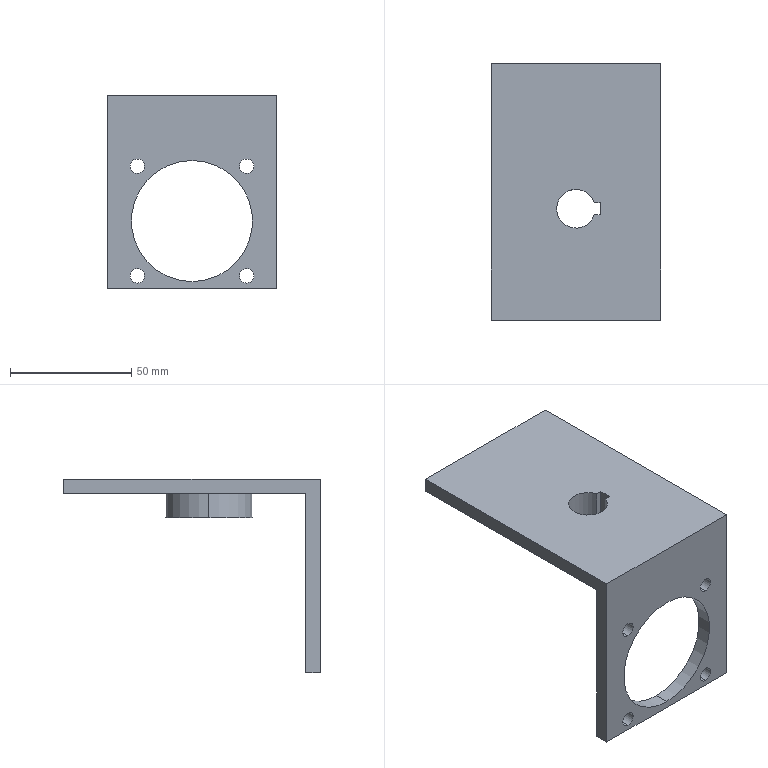Part | SolidWorks | features ICE 3, Cut 1, Extrusion 1 | 1 solid | 26 faces | box 70 x 106 x 80 mm | volume 69922 mm3 | cylinder 14 | plane 12 | commonest cylinder face diameters 6 x6 6.013 x2 16 x2 36 x2 50.018 x2
STEP:
#1=CARTESIAN_POINT('',(22.627,-46.,-71.627));
#2=VERTEX_POINT('',#1);
#3=CARTESIAN_POINT('',(22.627,-46.,-65.627));
#4=VERTEX_POINT('',#3);
#5=CARTESIAN_POINT('',(22.627,-46.,-68.627));
#6=DIRECTION('',(0.,1.,0.));
#7=DIRECTION('',(0.,0.,1.));
#8=AXIS2_PLACEMENT_3D('',#5,#6,#7);
#9=CIRCLE('',#8,3.);
#10=EDGE_CURVE('',#2,#4,#9,.T.);
#11=ORIENTED_EDGE('',*,*,#10,.F.);
#12=CARTESIAN_POINT('',(22.627,-40.,-71.627));
#13=VERTEX_POINT('',#12);
#14=CARTESIAN_POINT('',(22.627,-46.,-71.627));
#15=DIRECTION('',(0.,1.,0.));
#16=VECTOR('',#15,1000.);
#17=LINE('',#14,#16);
#18=EDGE_CURVE('',#2,#13,#17,.T.);
#19=ORIENTED_EDGE('',*,*,#18,.T.);
#20=CARTESIAN_POINT('',(22.627,-40.,-65.627));
#21=VERTEX_POINT('',#20);
#22=CARTESIAN_POINT('',(22.627,-40.,-68.627));
#23=DIRECTION('',(0.,1.,0.));
#24=DIRECTION('',(0.,0.,1.));
#25=AXIS2_PLACEMENT_3D('',#22,#23,#24);
#26=CIRCLE('',#25,3.);
#27=EDGE_CURVE('',#13,#21,#26,.T.);
#28=ORIENTED_EDGE('',*,*,#27,.T.);
#29=CARTESIAN_POINT('',(22.627,-46.,-65.627));
#30=DIRECTION('',(0.,1.,0.));
#31=VECTOR('',#30,1000.);
#32=LINE('',#29,#31);
#33=EDGE_CURVE('',#4,#21,#32,.T.);
#34=ORIENTED_EDGE('',*,*,#33,.F.);
#35=EDGE_LOOP('',(#11,#19,#28,#34));
#36=FACE_OUTER_BOUND('',#35,.T.);
#37=CARTESIAN_POINT('',(22.627,-46.,-68.627));
#38=DIRECTION('',(0.,1.,0.));
#39=DIRECTION('',(0.,0.,1.));
#40=AXIS2_PLACEMENT_3D('',#37,#38,#39);
#41=CYLINDRICAL_SURFACE('',#40,3.);
#42=ADVANCED_FACE('',(#36),#41,.F.);
#43=CARTESIAN_POINT('',(22.627,-46.,-26.373));
#44=VERTEX_POINT('',#43);
#45=CARTESIAN_POINT('',(22.627,-46.,-20.373));
#46=VERTEX_POINT('',#45);
#47=CARTESIAN_POINT('',(22.627,-46.,-23.373));
#48=DIRECTION('',(0.,1.,0.));
#49=DIRECTION('',(0.,0.,1.));
#50=AXIS2_PLACEMENT_3D('',#47,#48,#49);
#51=CIRCLE('',#50,3.);
#52=EDGE_CURVE('',#44,#46,#51,.T.);
#53=ORIENTED_EDGE('',*,*,#52,.F.);
#54=CARTESIAN_POINT('',(22.627,-40.,-26.373));
#55=VERTEX_POINT('',#54);
#56=CARTESIAN_POINT('',(22.627,-46.,-26.373));
#57=DIRECTION('',(0.,1.,0.));
#58=VECTOR('',#57,1000.);
#59=LINE('',#56,#58);
#60=EDGE_CURVE('',#44,#55,#59,.T.);
#61=ORIENTED_EDGE('',*,*,#60,.T.);
#62=CARTESIAN_POINT('',(22.627,-40.,-20.373));
#63=VERTEX_POINT('',#62);
#64=CARTESIAN_POINT('',(22.627,-40.,-23.373));
#65=DIRECTION('',(0.,1.,0.));
#66=DIRECTION('',(0.,0.,1.));
#67=AXIS2_PLACEMENT_3D('',#64,#65,#66);
#68=CIRCLE('',#67,3.);
#69=EDGE_CURVE('',#55,#63,#68,.T.);
#70=ORIENTED_EDGE('',*,*,#69,.T.);
#71=CARTESIAN_POINT('',(22.627,-46.,-20.373));
#72=DIRECTION('',(0.,1.,0.));
#73=VECTOR('',#72,1000.);
#74=LINE('',#71,#73);
#75=EDGE_CURVE('',#46,#63,#74,.T.);
#76=ORIENTED_EDGE('',*,*,#75,.F.);
#77=EDGE_LOOP('',(#53,#61,#70,#76));
#78=FACE_OUTER_BOUND('',#77,.T.);
#79=CARTESIAN_POINT('',(22.627,-46.,-23.373));
#80=DIRECTION('',(0.,1.,0.));
#81=DIRECTION('',(0.,0.,1.));
#82=AXIS2_PLACEMENT_3D('',#79,#80,#81);
#83=CYLINDRICAL_SURFACE('',#82,3.);
#84=ADVANCED_FACE('',(#78),#83,.F.);
#85=CARTESIAN_POINT('',(-0.009138,-46.,-71.009));
#86=VERTEX_POINT('',#85);
#87=CARTESIAN_POINT('',(-0.009138,-46.,-20.991));
#88=VERTEX_POINT('',#87);
#89=CARTESIAN_POINT('',(-0.009138,-46.,-46.));
#90=DIRECTION('',(0.,1.,0.));
#91=DIRECTION('',(0.,0.,1.));
#92=AXIS2_PLACEMENT_3D('',#89,#90,#91);
#93=CIRCLE('',#92,25.009);
#94=EDGE_CURVE('',#86,#88,#93,.T.);
#95=ORIENTED_EDGE('',*,*,#94,.F.);
#96=CARTESIAN_POINT('',(-0.009138,-40.,-71.009));
#97=VERTEX_POINT('',#96);
#98=CARTESIAN_POINT('',(-0.009138,-46.,-71.009));
#99=DIRECTION('',(0.,1.,0.));
#100=VECTOR('',#99,1000.);
#101=LINE('',#98,#100);
#102=EDGE_CURVE('',#86,#97,#101,.T.);
#103=ORIENTED_EDGE('',*,*,#102,.T.);
#104=CARTESIAN_POINT('',(-0.009138,-40.,-20.991));
#105=VERTEX_POINT('',#104);
#106=CARTESIAN_POINT('',(-0.009138,-40.,-46.));
#107=DIRECTION('',(0.,1.,0.));
#108=DIRECTION('',(0.,0.,1.));
#109=AXIS2_PLACEMENT_3D('',#106,#107,#108);
#110=CIRCLE('',#109,25.009);
#111=EDGE_CURVE('',#97,#105,#110,.T.);
#112=ORIENTED_EDGE('',*,*,#111,.T.);
#113=CARTESIAN_POINT('',(-0.009138,-46.,-20.991));
#114=DIRECTION('',(0.,1.,0.));
#115=VECTOR('',#114,1000.);
#116=LINE('',#113,#115);
#117=EDGE_CURVE('',#88,#105,#116,.T.);
#118=ORIENTED_EDGE('',*,*,#117,.F.);
#119=EDGE_LOOP('',(#95,#103,#112,#118));
#120=FACE_OUTER_BOUND('',#119,.T.);
#121=CARTESIAN_POINT('',(-0.009138,-46.,-46.));
#122=DIRECTION('',(0.,1.,0.));
#123=DIRECTION('',(0.,0.,1.));
#124=AXIS2_PLACEMENT_3D('',#121,#122,#123);
#125=CYLINDRICAL_SURFACE('',#124,25.009);
#126=ADVANCED_FACE('',(#120),#125,.F.);
#127=CARTESIAN_POINT('',(-22.627,-46.,-26.373));
#128=VERTEX_POINT('',#127);
#129=CARTESIAN_POINT('',(-22.627,-46.,-20.373));
#130=VERTEX_POINT('',#129);
#131=CARTESIAN_POINT('',(-22.627,-46.,-23.373));
#132=DIRECTION('',(0.,1.,0.));
#133=DIRECTION('',(0.,0.,1.));
#134=AXIS2_PLACEMENT_3D('',#131,#132,#133);
#135=CIRCLE('',#134,3.);
#136=EDGE_CURVE('',#128,#130,#135,.T.);
#137=ORIENTED_EDGE('',*,*,#136,.F.);
#138=CARTESIAN_POINT('',(-22.627,-40.,-26.373));
#139=VERTEX_POINT('',#138);
#140=CARTESIAN_POINT('',(-22.627,-46.,-26.373));
#141=DIRECTION('',(0.,1.,0.));
#142=VECTOR('',#141,1000.);
#143=LINE('',#140,#142);
#144=EDGE_CURVE('',#128,#139,#143,.T.);
#145=ORIENTED_EDGE('',*,*,#144,.T.);
#146=CARTESIAN_POINT('',(-22.627,-40.,-20.373));
#147=VERTEX_POINT('',#146);
#148=CARTESIAN_POINT('',(-22.627,-40.,-23.373));
#149=DIRECTION('',(0.,1.,0.));
#150=DIRECTION('',(0.,0.,1.));
#151=AXIS2_PLACEMENT_3D('',#148,#149,#150);
#152=CIRCLE('',#151,3.);
#153=EDGE_CURVE('',#139,#147,#152,.T.);
#154=ORIENTED_EDGE('',*,*,#153,.T.);
#155=CARTESIAN_POINT('',(-22.627,-46.,-20.373));
#156=DIRECTION('',(0.,1.,0.));
#157=VECTOR('',#156,1000.);
#158=LINE('',#155,#157);
#159=EDGE_CURVE('',#130,#147,#158,.T.);
#160=ORIENTED_EDGE('',*,*,#159,.F.);
#161=EDGE_LOOP('',(#137,#145,#154,#160));
#162=FACE_OUTER_BOUND('',#161,.T.);
#163=CARTESIAN_POINT('',(-22.627,-46.,-23.373));
#164=DIRECTION('',(0.,1.,0.));
#165=DIRECTION('',(0.,0.,1.));
#166=AXIS2_PLACEMENT_3D('',#163,#164,#165);
#167=CYLINDRICAL_SURFACE('',#166,3.);
#168=ADVANCED_FACE('',(#162),#167,.F.);
#169=CARTESIAN_POINT('',(-22.627,-46.,-71.634));
#170=VERTEX_POINT('',#169);
#171=CARTESIAN_POINT('',(-22.627,-46.,-65.621));
#172=VERTEX_POINT('',#171);
#173=CARTESIAN_POINT('',(-22.627,-46.,-68.627));
#174=DIRECTION('',(0.,1.,0.));
#175=DIRECTION('',(0.,0.,1.));
#176=AXIS2_PLACEMENT_3D('',#173,#174,#175);
#177=CIRCLE('',#176,3.006);
#178=EDGE_CURVE('',#170,#172,#177,.T.);
#179=ORIENTED_EDGE('',*,*,#178,.F.);
#180=CARTESIAN_POINT('',(-22.627,-40.,-71.634));
#181=VERTEX_POINT('',#180);
#182=CARTESIAN_POINT('',(-22.627,-46.,-71.634));
#183=DIRECTION('',(0.,1.,0.));
#184=VECTOR('',#183,1000.);
#185=LINE('',#182,#184);
#186=EDGE_CURVE('',#170,#181,#185,.T.);
#187=ORIENTED_EDGE('',*,*,#186,.T.);
#188=CARTESIAN_POINT('',(-22.627,-40.,-65.621));
#189=VERTEX_POINT('',#188);
#190=CARTESIAN_POINT('',(-22.627,-40.,-68.627));
#191=DIRECTION('',(0.,1.,0.));
#192=DIRECTION('',(0.,0.,1.));
#193=AXIS2_PLACEMENT_3D('',#190,#191,#192);
#194=CIRCLE('',#193,3.006);
#195=EDGE_CURVE('',#181,#189,#194,.T.);
#196=ORIENTED_EDGE('',*,*,#195,.T.);
#197=CARTESIAN_POINT('',(-22.627,-46.,-65.621));
#198=DIRECTION('',(0.,1.,0.));
#199=VECTOR('',#198,1000.);
#200=LINE('',#197,#199);
#201=EDGE_CURVE('',#172,#189,#200,.T.);
#202=ORIENTED_EDGE('',*,*,#201,.F.);
#203=EDGE_LOOP('',(#179,#187,#196,#202));
#204=FACE_OUTER_BOUND('',#203,.T.);
#205=CARTESIAN_POINT('',(-22.627,-46.,-68.627));
#206=DIRECTION('',(0.,1.,0.));
#207=DIRECTION('',(0.,0.,1.));
#208=AXIS2_PLACEMENT_3D('',#205,#206,#207);
#209=CYLINDRICAL_SURFACE('',#208,3.006);
#210=ADVANCED_FACE('',(#204),#209,.F.);
#211=CARTESIAN_POINT('',(-18.,0.,-10.));
#212=VERTEX_POINT('',#211);
#213=CARTESIAN_POINT('',(18.,0.,-10.));
#214=VERTEX_POINT('',#213);
#215=CARTESIAN_POINT('',(0.,0.,-10.));
#216=DIRECTION('',(0.,0.,-1.));
#217=DIRECTION('',(-1.,0.,0.));
#218=AXIS2_PLACEMENT_3D('',#215,#216,#217);
#219=CIRCLE('',#218,18.);
#220=EDGE_CURVE('',#212,#214,#219,.T.);
#221=ORIENTED_EDGE('',*,*,#220,.F.);
#222=CARTESIAN_POINT('',(-18.,0.,0.));
#223=VERTEX_POINT('',#222);
#224=CARTESIAN_POINT('',(-18.,0.,-10.));
#225=DIRECTION('',(0.,0.,1.));
#226=VECTOR('',#225,1000.);
#227=LINE('',#224,#226);
#228=EDGE_CURVE('',#212,#223,#227,.T.);
#229=ORIENTED_EDGE('',*,*,#228,.T.);
#230=CARTESIAN_POINT('',(18.,0.,0.));
#231=VERTEX_POINT('',#230);
#232=CARTESIAN_POINT('',(0.,0.,0.));
#233=DIRECTION('',(0.,0.,-1.));
#234=DIRECTION('',(1.,0.,0.));
#235=AXIS2_PLACEMENT_3D('',#232,#233,#234);
#236=CIRCLE('',#235,18.);
#237=EDGE_CURVE('',#223,#231,#236,.T.);
#238=ORIENTED_EDGE('',*,*,#237,.T.);
#239=CARTESIAN_POINT('',(18.,0.,-10.));
#240=DIRECTION('',(0.,0.,1.));
#241=VECTOR('',#240,1000.);
#242=LINE('',#239,#241);
#243=EDGE_CURVE('',#214,#231,#242,.T.);
#244=ORIENTED_EDGE('',*,*,#243,.F.);
#245=EDGE_LOOP('',(#221,#229,#238,#244));
#246=FACE_OUTER_BOUND('',#245,.T.);
#247=CARTESIAN_POINT('',(0.,0.,-10.));
#248=DIRECTION('',(0.,0.,1.));
#249=DIRECTION('',(1.,0.,0.));
#250=AXIS2_PLACEMENT_3D('',#247,#248,#249);
#251=CYLINDRICAL_SURFACE('',#250,18.);
#252=ADVANCED_FACE('',(#246),#251,.T.);
#253=CARTESIAN_POINT('',(7.599,2.5,6.));
#254=VERTEX_POINT('',#253);
#255=CARTESIAN_POINT('',(-8.,0.,6.));
#256=VERTEX_POINT('',#255);
#257=CARTESIAN_POINT('',(0.,0.,6.));
#258=DIRECTION('',(0.,0.,1.));
#259=DIRECTION('',(1.,0.,0.));
#260=AXIS2_PLACEMENT_3D('',#257,#258,#259);
#261=CIRCLE('',#260,8.);
#262=EDGE_CURVE('',#254,#256,#261,.T.);
#263=ORIENTED_EDGE('',*,*,#262,.T.);
#264=CARTESIAN_POINT('',(-8.,0.,-10.));
#265=VERTEX_POINT('',#264);
#266=CARTESIAN_POINT('',(-8.,0.,6.));
#267=DIRECTION('',(0.,0.,-1.));
#268=VECTOR('',#267,1000.);
#269=LINE('',#266,#268);
#270=EDGE_CURVE('',#256,#265,#269,.T.);
#271=ORIENTED_EDGE('',*,*,#270,.T.);
#272=CARTESIAN_POINT('',(7.599,2.5,-10.));
#273=VERTEX_POINT('',#272);
#274=CARTESIAN_POINT('',(0.,0.,-10.));
#275=DIRECTION('',(0.,0.,-1.));
#276=DIRECTION('',(-1.,0.,0.));
#277=AXIS2_PLACEMENT_3D('',#274,#275,#276);
#278=CIRCLE('',#277,8.);
#279=EDGE_CURVE('',#265,#273,#278,.T.);
#280=ORIENTED_EDGE('',*,*,#279,.T.);
#281=CARTESIAN_POINT('',(7.599,2.5,6.));
#282=DIRECTION('',(0.,0.,-1.));
#283=VECTOR('',#282,1000.);
#284=LINE('',#281,#283);
#285=EDGE_CURVE('',#254,#273,#284,.T.);
#286=ORIENTED_EDGE('',*,*,#285,.F.);
#287=EDGE_LOOP('',(#263,#271,#280,#286));
#288=FACE_OUTER_BOUND('',#287,.T.);
#289=CARTESIAN_POINT('',(0.,0.,6.));
#290=DIRECTION('',(0.,0.,-1.));
#291=DIRECTION('',(-1.,0.,0.));
#292=AXIS2_PLACEMENT_3D('',#289,#290,#291);
#293=CYLINDRICAL_SURFACE('',#292,8.);
#294=ADVANCED_FACE('',(#288),#293,.F.);
#295=CARTESIAN_POINT('',(-35.,60.,0.));
#296=VERTEX_POINT('',#295);
#297=CARTESIAN_POINT('',(-35.,-40.,0.));
#298=VERTEX_POINT('',#297);
#299=CARTESIAN_POINT('',(-35.,60.,0.));
#300=DIRECTION('',(0.,-1.,0.));
#301=VECTOR('',#300,1000.);
#302=LINE('',#299,#301);
#303=EDGE_CURVE('',#296,#298,#302,.T.);
#304=ORIENTED_EDGE('',*,*,#303,.F.);
#305=CARTESIAN_POINT('',(35.,60.,0.));
#306=VERTEX_POINT('',#305);
#307=CARTESIAN_POINT('',(-35.,60.,0.));
#308=DIRECTION('',(-1.,0.,0.));
#309=VECTOR('',#308,1000.);
#310=LINE('',#307,#309);
#311=EDGE_CURVE('',#306,#296,#310,.T.);
#312=ORIENTED_EDGE('',*,*,#311,.F.);
#313=CARTESIAN_POINT('',(35.,-40.,0.));
#314=VERTEX_POINT('',#313);
#315=CARTESIAN_POINT('',(35.,60.,0.));
#316=DIRECTION('',(0.,1.,0.));
#317=VECTOR('',#316,1000.);
#318=LINE('',#315,#317);
#319=EDGE_CURVE('',#314,#306,#318,.T.);
#320=ORIENTED_EDGE('',*,*,#319,.F.);
#321=CARTESIAN_POINT('',(-35.,-40.,0.));
#322=DIRECTION('',(1.,0.,0.));
#323=VECTOR('',#322,1000.);
#324=LINE('',#321,#323);
#325=EDGE_CURVE('',#298,#314,#324,.T.);
#326=ORIENTED_EDGE('',*,*,#325,.F.);
#327=EDGE_LOOP('',(#304,#312,#320,#326));
#328=FACE_OUTER_BOUND('',#327,.T.);
#329=CARTESIAN_POINT('',(0.,0.,0.));
#330=DIRECTION('',(0.,0.,-1.));
#331=DIRECTION('',(1.,0.,0.));
#332=AXIS2_PLACEMENT_3D('',#329,#330,#331);
#333=CIRCLE('',#332,18.);
#334=EDGE_CURVE('',#231,#223,#333,.T.);
#335=ORIENTED_EDGE('',*,*,#334,.F.);
#336=ORIENTED_EDGE('',*,*,#237,.F.);
#337=EDGE_LOOP('',(#335,#336));
#338=FACE_BOUND('',#337,.T.);
#339=CARTESIAN_POINT('',(0.,0.,0.));
#340=DIRECTION('',(0.,0.,1.));
#341=DIRECTION('',(1.,0.,0.));
#342=AXIS2_PLACEMENT_3D('',#339,#340,#341);
#343=PLANE('',#342);
#344=ADVANCED_FACE('',(#328,#338),#343,.F.);
#345=CARTESIAN_POINT('',(10.,2.5,6.));
#346=VERTEX_POINT('',#345);
#347=CARTESIAN_POINT('',(10.,2.5,6.));
#348=DIRECTION('',(1.,0.,0.));
#349=VECTOR('',#348,1000.);
#350=LINE('',#347,#349);
#351=EDGE_CURVE('',#254,#346,#350,.T.);
#352=ORIENTED_EDGE('',*,*,#351,.T.);
#353=CARTESIAN_POINT('',(10.,-2.5,6.));
#354=VERTEX_POINT('',#353);
#355=CARTESIAN_POINT('',(10.,2.5,6.));
#356=DIRECTION('',(0.,-1.,0.));
#357=VECTOR('',#356,1000.);
#358=LINE('',#355,#357);
#359=EDGE_CURVE('',#346,#354,#358,.T.);
#360=ORIENTED_EDGE('',*,*,#359,.T.);
#361=CARTESIAN_POINT('',(7.599,-2.5,6.));
#362=VERTEX_POINT('',#361);
#363=CARTESIAN_POINT('',(10.,-2.5,6.));
#364=DIRECTION('',(-1.,0.,0.));
#365=VECTOR('',#364,1000.);
#366=LINE('',#363,#365);
#367=EDGE_CURVE('',#354,#362,#366,.T.);
#368=ORIENTED_EDGE('',*,*,#367,.T.);
#369=CARTESIAN_POINT('',(0.,0.,6.));
#370=DIRECTION('',(0.,0.,1.));
#371=DIRECTION('',(1.,0.,0.));
#372=AXIS2_PLACEMENT_3D('',#369,#370,#371);
#373=CIRCLE('',#372,8.);
#374=EDGE_CURVE('',#256,#362,#373,.T.);
#375=ORIENTED_EDGE('',*,*,#374,.F.);
#376=ORIENTED_EDGE('',*,*,#262,.F.);
#377=EDGE_LOOP('',(#352,#360,#368,#375,#376));
#378=FACE_BOUND('',#377,.T.);
#379=CARTESIAN_POINT('',(-35.,60.,6.));
#380=VERTEX_POINT('',#379);
#381=CARTESIAN_POINT('',(-35.,-46.,6.));
#382=VERTEX_POINT('',#381);
#383=CARTESIAN_POINT('',(-35.,60.,6.));
#384=DIRECTION('',(0.,-1.,0.));
#385=VECTOR('',#384,1000.);
#386=LINE('',#383,#385);
#387=EDGE_CURVE('',#380,#382,#386,.T.);
#388=ORIENTED_EDGE('',*,*,#387,.T.);
#389=CARTESIAN_POINT('',(35.,-46.,6.));
#390=VERTEX_POINT('',#389);
#391=CARTESIAN_POINT('',(-35.,-46.,6.));
#392=DIRECTION('',(-1.,0.,0.));
#393=VECTOR('',#392,1000.);
#394=LINE('',#391,#393);
#395=EDGE_CURVE('',#390,#382,#394,.T.);
#396=ORIENTED_EDGE('',*,*,#395,.F.);
#397=CARTESIAN_POINT('',(35.,60.,6.));
#398=VERTEX_POINT('',#397);
#399=CARTESIAN_POINT('',(35.,60.,6.));
#400=DIRECTION('',(0.,1.,0.));
#401=VECTOR('',#400,1000.);
#402=LINE('',#399,#401);
#403=EDGE_CURVE('',#390,#398,#402,.T.);
#404=ORIENTED_EDGE('',*,*,#403,.T.);
#405=CARTESIAN_POINT('',(-35.,60.,6.));
#406=DIRECTION('',(-1.,0.,0.));
#407=VECTOR('',#406,1000.);
#408=LINE('',#405,#407);
#409=EDGE_CURVE('',#398,#380,#408,.T.);
#410=ORIENTED_EDGE('',*,*,#409,.T.);
#411=EDGE_LOOP('',(#388,#396,#404,#410));
#412=FACE_OUTER_BOUND('',#411,.T.);
#413=CARTESIAN_POINT('',(0.,0.,6.));
#414=DIRECTION('',(0.,0.,1.));
#415=DIRECTION('',(1.,0.,0.));
#416=AXIS2_PLACEMENT_3D('',#413,#414,#415);
#417=PLANE('',#416);
#418=ADVANCED_FACE('',(#378,#412),#417,.T.);
#419=ORIENTED_EDGE('',*,*,#303,.T.);
#420=CARTESIAN_POINT('',(-35.,-40.,-74.));
#421=VERTEX_POINT('',#420);
#422=CARTESIAN_POINT('',(-35.,-40.,6.));
#423=DIRECTION('',(0.,0.,-1.));
#424=VECTOR('',#423,1000.);
#425=LINE('',#422,#424);
#426=EDGE_CURVE('',#298,#421,#425,.T.);
#427=ORIENTED_EDGE('',*,*,#426,.T.);
#428=CARTESIAN_POINT('',(-35.,-46.,-74.));
#429=VERTEX_POINT('',#428);
#430=CARTESIAN_POINT('',(-35.,-46.,-74.));
#431=DIRECTION('',(0.,1.,0.));
#432=VECTOR('',#431,1000.);
#433=LINE('',#430,#432);
#434=EDGE_CURVE('',#429,#421,#433,.T.);
#435=ORIENTED_EDGE('',*,*,#434,.F.);
#436=CARTESIAN_POINT('',(-35.,-46.,6.));
#437=DIRECTION('',(0.,0.,-1.));
#438=VECTOR('',#437,1000.);
#439=LINE('',#436,#438);
#440=EDGE_CURVE('',#382,#429,#439,.T.);
#441=ORIENTED_EDGE('',*,*,#440,.F.);
#442=ORIENTED_EDGE('',*,*,#387,.F.);
#443=CARTESIAN_POINT('',(-35.,60.,6.));
#444=DIRECTION('',(0.,0.,-1.));
#445=VECTOR('',#444,1000.);
#446=LINE('',#443,#445);
#447=EDGE_CURVE('',#380,#296,#446,.T.);
#448=ORIENTED_EDGE('',*,*,#447,.T.);
#449=EDGE_LOOP('',(#419,#427,#435,#441,#442,#448));
#450=FACE_OUTER_BOUND('',#449,.T.);
#451=CARTESIAN_POINT('',(-35.,60.,6.));
#452=DIRECTION('',(1.,0.,0.));
#453=DIRECTION('',(0.,1.,0.));
#454=AXIS2_PLACEMENT_3D('',#451,#452,#453);
#455=PLANE('',#454);
#456=ADVANCED_FACE('',(#450),#455,.F.);
#457=ORIENTED_EDGE('',*,*,#319,.T.);
#458=CARTESIAN_POINT('',(35.,60.,6.));
#459=DIRECTION('',(0.,0.,-1.));
#460=VECTOR('',#459,1000.);
#461=LINE('',#458,#460);
#462=EDGE_CURVE('',#398,#306,#461,.T.);
#463=ORIENTED_EDGE('',*,*,#462,.F.);
#464=ORIENTED_EDGE('',*,*,#403,.F.);
#465=CARTESIAN_POINT('',(35.,-46.,-74.));
#466=VERTEX_POINT('',#465);
#467=CARTESIAN_POINT('',(35.,-46.,6.));
#468=DIRECTION('',(0.,0.,1.));
#469=VECTOR('',#468,1000.);
#470=LINE('',#467,#469);
#471=EDGE_CURVE('',#466,#390,#470,.T.);
#472=ORIENTED_EDGE('',*,*,#471,.F.);
#473=CARTESIAN_POINT('',(35.,-40.,-74.));
#474=VERTEX_POINT('',#473);
#475=CARTESIAN_POINT('',(35.,-46.,-74.));
#476=DIRECTION('',(0.,1.,0.));
#477=VECTOR('',#476,1000.);
#478=LINE('',#475,#477);
#479=EDGE_CURVE('',#466,#474,#478,.T.);
#480=ORIENTED_EDGE('',*,*,#479,.T.);
#481=CARTESIAN_POINT('',(35.,-40.,6.));
#482=DIRECTION('',(0.,0.,1.));
#483=VECTOR('',#482,1000.);
#484=LINE('',#481,#483);
#485=EDGE_CURVE('',#474,#314,#484,.T.);
#486=ORIENTED_EDGE('',*,*,#485,.T.);
#487=EDGE_LOOP('',(#457,#463,#464,#472,#480,#486));
#488=FACE_OUTER_BOUND('',#487,.T.);
#489=CARTESIAN_POINT('',(35.,60.,6.));
#490=DIRECTION('',(-1.,0.,0.));
#491=DIRECTION('',(0.,-1.,0.));
#492=AXIS2_PLACEMENT_3D('',#489,#490,#491);
#493=PLANE('',#492);
#494=ADVANCED_FACE('',(#488),#493,.F.);
#495=ORIENTED_EDGE('',*,*,#311,.T.);
#496=ORIENTED_EDGE('',*,*,#447,.F.);
#497=ORIENTED_EDGE('',*,*,#409,.F.);
#498=ORIENTED_EDGE('',*,*,#462,.T.);
#499=EDGE_LOOP('',(#495,#496,#497,#498));
#500=FACE_OUTER_BOUND('',#499,.T.);
#501=CARTESIAN_POINT('',(-35.,60.,6.));
#502=DIRECTION('',(0.,-1.,0.));
#503=DIRECTION('',(0.,0.,-1.));
#504=AXIS2_PLACEMENT_3D('',#501,#502,#503);
#505=PLANE('',#504);
#506=ADVANCED_FACE('',(#500),#505,.F.);
#507=ORIENTED_EDGE('',*,*,#270,.F.);
#508=ORIENTED_EDGE('',*,*,#374,.T.);
#509=CARTESIAN_POINT('',(7.599,-2.5,-10.));
#510=VERTEX_POINT('',#509);
#511=CARTESIAN_POINT('',(7.599,-2.5,6.));
#512=DIRECTION('',(0.,0.,1.));
#513=VECTOR('',#512,1000.);
#514=LINE('',#511,#513);
#515=EDGE_CURVE('',#510,#362,#514,.T.);
#516=ORIENTED_EDGE('',*,*,#515,.F.);
#517=CARTESIAN_POINT('',(0.,0.,-10.));
#518=DIRECTION('',(0.,0.,-1.));
#519=DIRECTION('',(-1.,0.,0.));
#520=AXIS2_PLACEMENT_3D('',#517,#518,#519);
#521=CIRCLE('',#520,8.);
#522=EDGE_CURVE('',#510,#265,#521,.T.);
#523=ORIENTED_EDGE('',*,*,#522,.T.);
#524=EDGE_LOOP('',(#507,#508,#516,#523));
#525=FACE_OUTER_BOUND('',#524,.T.);
#526=CARTESIAN_POINT('',(0.,0.,6.));
#527=DIRECTION('',(0.,0.,-1.));
#528=DIRECTION('',(-1.,0.,0.));
#529=AXIS2_PLACEMENT_3D('',#526,#527,#528);
#530=CYLINDRICAL_SURFACE('',#529,8.);
#531=ADVANCED_FACE('',(#525),#530,.F.);
#532=CARTESIAN_POINT('',(10.,2.5,-10.));
#533=VERTEX_POINT('',#532);
#534=CARTESIAN_POINT('',(0.,2.5,-10.));
#535=DIRECTION('',(1.,0.,0.));
#536=VECTOR('',#535,1000.);
#537=LINE('',#534,#536);
#538=EDGE_CURVE('',#273,#533,#537,.T.);
#539=ORIENTED_EDGE('',*,*,#538,.F.);
#540=ORIENTED_EDGE('',*,*,#279,.F.);
#541=ORIENTED_EDGE('',*,*,#522,.F.);
#542=CARTESIAN_POINT('',(10.,-2.5,-10.));
#543=VERTEX_POINT('',#542);
#544=CARTESIAN_POINT('',(10.,-2.5,-10.));
#545=DIRECTION('',(-1.,0.,0.));
#546=VECTOR('',#545,1000.);
#547=LINE('',#544,#546);
#548=EDGE_CURVE('',#543,#510,#547,.T.);
#549=ORIENTED_EDGE('',*,*,#548,.F.);
#550=CARTESIAN_POINT('',(10.,2.5,-10.));
#551=DIRECTION('',(0.,-1.,0.));
#552=VECTOR('',#551,1000.);
#553=LINE('',#550,#552);
#554=EDGE_CURVE('',#533,#543,#553,.T.);
#555=ORIENTED_EDGE('',*,*,#554,.F.);
#556=EDGE_LOOP('',(#539,#540,#541,#549,#555));
#557=FACE_BOUND('',#556,.T.);
#558=CARTESIAN_POINT('',(0.,0.,-10.));
#559=DIRECTION('',(0.,0.,-1.));
#560=DIRECTION('',(-1.,0.,0.));
#561=AXIS2_PLACEMENT_3D('',#558,#559,#560);
#562=CIRCLE('',#561,18.);
#563=EDGE_CURVE('',#214,#212,#562,.T.);
#564=ORIENTED_EDGE('',*,*,#563,.T.);
#565=ORIENTED_EDGE('',*,*,#220,.T.);
#566=EDGE_LOOP('',(#564,#565));
#567=FACE_OUTER_BOUND('',#566,.T.);
#568=CARTESIAN_POINT('',(0.,0.,-10.));
#569=DIRECTION('',(0.,0.,-1.));
#570=DIRECTION('',(-1.,0.,0.));
#571=AXIS2_PLACEMENT_3D('',#568,#569,#570);
#572=PLANE('',#571);
#573=ADVANCED_FACE('',(#557,#567),#572,.T.);
#574=ORIENTED_EDGE('',*,*,#228,.F.);
#575=ORIENTED_EDGE('',*,*,#563,.F.);
#576=ORIENTED_EDGE('',*,*,#243,.T.);
#577=ORIENTED_EDGE('',*,*,#334,.T.);
#578=EDGE_LOOP('',(#574,#575,#576,#577));
#579=FACE_OUTER_BOUND('',#578,.T.);
#580=CARTESIAN_POINT('',(0.,0.,-10.));
#581=DIRECTION('',(0.,0.,1.));
#582=DIRECTION('',(1.,0.,0.));
#583=AXIS2_PLACEMENT_3D('',#580,#581,#582);
#584=CYLINDRICAL_SURFACE('',#583,18.);
#585=ADVANCED_FACE('',(#579),#584,.T.);
#586=CARTESIAN_POINT('',(22.627,-40.,-68.627));
#587=DIRECTION('',(0.,1.,0.));
#588=DIRECTION('',(0.,0.,1.));
#589=AXIS2_PLACEMENT_3D('',#586,#587,#588);
#590=CIRCLE('',#589,3.);
#591=EDGE_CURVE('',#21,#13,#590,.T.);
#592=ORIENTED_EDGE('',*,*,#591,.F.);
#593=ORIENTED_EDGE('',*,*,#27,.F.);
#594=EDGE_LOOP('',(#592,#593));
#595=FACE_BOUND('',#594,.T.);
#596=CARTESIAN_POINT('',(22.627,-40.,-23.373));
#597=DIRECTION('',(0.,1.,0.));
#598=DIRECTION('',(0.,0.,1.));
#599=AXIS2_PLACEMENT_3D('',#596,#597,#598);
#600=CIRCLE('',#599,3.);
#601=EDGE_CURVE('',#63,#55,#600,.T.);
#602=ORIENTED_EDGE('',*,*,#601,.F.);
#603=ORIENTED_EDGE('',*,*,#69,.F.);
#604=EDGE_LOOP('',(#602,#603));
#605=FACE_BOUND('',#604,.T.);
#606=CARTESIAN_POINT('',(-0.009138,-40.,-46.));
#607=DIRECTION('',(0.,1.,0.));
#608=DIRECTION('',(0.,0.,1.));
#609=AXIS2_PLACEMENT_3D('',#606,#607,#608);
#610=CIRCLE('',#609,25.009);
#611=EDGE_CURVE('',#105,#97,#610,.T.);
#612=ORIENTED_EDGE('',*,*,#611,.F.);
#613=ORIENTED_EDGE('',*,*,#111,.F.);
#614=EDGE_LOOP('',(#612,#613));
#615=FACE_BOUND('',#614,.T.);
#616=CARTESIAN_POINT('',(-22.627,-40.,-23.373));
#617=DIRECTION('',(0.,1.,0.));
#618=DIRECTION('',(0.,0.,1.));
#619=AXIS2_PLACEMENT_3D('',#616,#617,#618);
#620=CIRCLE('',#619,3.);
#621=EDGE_CURVE('',#147,#139,#620,.T.);
#622=ORIENTED_EDGE('',*,*,#621,.F.);
#623=ORIENTED_EDGE('',*,*,#153,.F.);
#624=EDGE_LOOP('',(#622,#623));
#625=FACE_BOUND('',#624,.T.);
#626=CARTESIAN_POINT('',(-22.627,-40.,-68.627));
#627=DIRECTION('',(0.,1.,0.));
#628=DIRECTION('',(0.,0.,1.));
#629=AXIS2_PLACEMENT_3D('',#626,#627,#628);
#630=CIRCLE('',#629,3.006);
#631=EDGE_CURVE('',#189,#181,#630,.T.);
#632=ORIENTED_EDGE('',*,*,#631,.F.);
#633=ORIENTED_EDGE('',*,*,#195,.F.);
#634=EDGE_LOOP('',(#632,#633));
#635=FACE_BOUND('',#634,.T.);
#636=ORIENTED_EDGE('',*,*,#426,.F.);
#637=ORIENTED_EDGE('',*,*,#325,.T.);
#638=ORIENTED_EDGE('',*,*,#485,.F.);
#639=CARTESIAN_POINT('',(-35.,-40.,-74.));
#640=DIRECTION('',(1.,0.,0.));
#641=VECTOR('',#640,1000.);
#642=LINE('',#639,#641);
#643=EDGE_CURVE('',#421,#474,#642,.T.);
#644=ORIENTED_EDGE('',*,*,#643,.F.);
#645=EDGE_LOOP('',(#636,#637,#638,#644));
#646=FACE_OUTER_BOUND('',#645,.T.);
#647=CARTESIAN_POINT('',(0.,-40.,0.));
#648=DIRECTION('',(0.,-1.,0.));
#649=DIRECTION('',(0.,0.,-1.));
#650=AXIS2_PLACEMENT_3D('',#647,#648,#649);
#651=PLANE('',#650);
#652=ADVANCED_FACE('',(#595,#605,#615,#625,#635,#646),#651,.F.);
#653=ORIENTED_EDGE('',*,*,#643,.T.);
#654=ORIENTED_EDGE('',*,*,#479,.F.);
#655=CARTESIAN_POINT('',(-35.,-46.,-74.));
#656=DIRECTION('',(1.,0.,0.));
#657=VECTOR('',#656,1000.);
#658=LINE('',#655,#657);
#659=EDGE_CURVE('',#429,#466,#658,.T.);
#660=ORIENTED_EDGE('',*,*,#659,.F.);
#661=ORIENTED_EDGE('',*,*,#434,.T.);
#662=EDGE_LOOP('',(#653,#654,#660,#661));
#663=FACE_OUTER_BOUND('',#662,.T.);
#664=CARTESIAN_POINT('',(-35.,-46.,-74.));
#665=DIRECTION('',(0.,0.,1.));
#666=DIRECTION('',(1.,0.,0.));
#667=AXIS2_PLACEMENT_3D('',#664,#665,#666);
#668=PLANE('',#667);
#669=ADVANCED_FACE('',(#663),#668,.F.);
#670=CARTESIAN_POINT('',(22.627,-46.,-68.627));
#671=DIRECTION('',(0.,1.,0.));
#672=DIRECTION('',(0.,0.,1.));
#673=AXIS2_PLACEMENT_3D('',#670,#671,#672);
#674=CIRCLE('',#673,3.);
#675=EDGE_CURVE('',#4,#2,#674,.T.);
#676=ORIENTED_EDGE('',*,*,#675,.T.);
#677=ORIENTED_EDGE('',*,*,#10,.T.);
#678=EDGE_LOOP('',(#676,#677));
#679=FACE_BOUND('',#678,.T.);
#680=CARTESIAN_POINT('',(22.627,-46.,-23.373));
#681=DIRECTION('',(0.,1.,0.));
#682=DIRECTION('',(0.,0.,1.));
#683=AXIS2_PLACEMENT_3D('',#680,#681,#682);
#684=CIRCLE('',#683,3.);
#685=EDGE_CURVE('',#46,#44,#684,.T.);
#686=ORIENTED_EDGE('',*,*,#685,.T.);
#687=ORIENTED_EDGE('',*,*,#52,.T.);
#688=EDGE_LOOP('',(#686,#687));
#689=FACE_BOUND('',#688,.T.);
#690=CARTESIAN_POINT('',(-0.009138,-46.,-46.));
#691=DIRECTION('',(0.,1.,0.));
#692=DIRECTION('',(0.,0.,1.));
#693=AXIS2_PLACEMENT_3D('',#690,#691,#692);
#694=CIRCLE('',#693,25.009);
#695=EDGE_CURVE('',#88,#86,#694,.T.);
#696=ORIENTED_EDGE('',*,*,#695,.T.);
#697=ORIENTED_EDGE('',*,*,#94,.T.);
#698=EDGE_LOOP('',(#696,#697));
#699=FACE_BOUND('',#698,.T.);
#700=CARTESIAN_POINT('',(-22.627,-46.,-23.373));
#701=DIRECTION('',(0.,1.,0.));
#702=DIRECTION('',(0.,0.,1.));
#703=AXIS2_PLACEMENT_3D('',#700,#701,#702);
#704=CIRCLE('',#703,3.);
#705=EDGE_CURVE('',#130,#128,#704,.T.);
#706=ORIENTED_EDGE('',*,*,#705,.T.);
#707=ORIENTED_EDGE('',*,*,#136,.T.);
#708=EDGE_LOOP('',(#706,#707));
#709=FACE_BOUND('',#708,.T.);
#710=CARTESIAN_POINT('',(-22.627,-46.,-68.627));
#711=DIRECTION('',(0.,1.,0.));
#712=DIRECTION('',(0.,0.,1.));
#713=AXIS2_PLACEMENT_3D('',#710,#711,#712);
#714=CIRCLE('',#713,3.006);
#715=EDGE_CURVE('',#172,#170,#714,.T.);
#716=ORIENTED_EDGE('',*,*,#715,.T.);
#717=ORIENTED_EDGE('',*,*,#178,.T.);
#718=EDGE_LOOP('',(#716,#717));
#719=FACE_BOUND('',#718,.T.);
#720=ORIENTED_EDGE('',*,*,#440,.T.);
#721=ORIENTED_EDGE('',*,*,#659,.T.);
#722=ORIENTED_EDGE('',*,*,#471,.T.);
#723=ORIENTED_EDGE('',*,*,#395,.T.);
#724=EDGE_LOOP('',(#720,#721,#722,#723));
#725=FACE_OUTER_BOUND('',#724,.T.);
#726=CARTESIAN_POINT('',(0.,-46.,0.));
#727=DIRECTION('',(0.,-1.,0.));
#728=DIRECTION('',(0.,0.,-1.));
#729=AXIS2_PLACEMENT_3D('',#726,#727,#728);
#730=PLANE('',#729);
#731=ADVANCED_FACE('',(#679,#689,#699,#709,#719,#725),#730,.T.);
#732=ORIENTED_EDGE('',*,*,#554,.T.);
#733=CARTESIAN_POINT('',(10.,-2.5,6.));
#734=DIRECTION('',(0.,0.,-1.));
#735=VECTOR('',#734,1000.);
#736=LINE('',#733,#735);
#737=EDGE_CURVE('',#354,#543,#736,.T.);
#738=ORIENTED_EDGE('',*,*,#737,.F.);
#739=ORIENTED_EDGE('',*,*,#359,.F.);
#740=CARTESIAN_POINT('',(10.,2.5,6.));
#741=DIRECTION('',(0.,0.,-1.));
#742=VECTOR('',#741,1000.);
#743=LINE('',#740,#742);
#744=EDGE_CURVE('',#346,#533,#743,.T.);
#745=ORIENTED_EDGE('',*,*,#744,.T.);
#746=EDGE_LOOP('',(#732,#738,#739,#745));
#747=FACE_OUTER_BOUND('',#746,.T.);
#748=CARTESIAN_POINT('',(10.,2.5,6.));
#749=DIRECTION('',(1.,0.,0.));
#750=DIRECTION('',(0.,1.,0.));
#751=AXIS2_PLACEMENT_3D('',#748,#749,#750);
#752=PLANE('',#751);
#753=ADVANCED_FACE('',(#747),#752,.F.);
#754=ORIENTED_EDGE('',*,*,#285,.T.);
#755=ORIENTED_EDGE('',*,*,#538,.T.);
#756=ORIENTED_EDGE('',*,*,#744,.F.);
#757=ORIENTED_EDGE('',*,*,#351,.F.);
#758=EDGE_LOOP('',(#754,#755,#756,#757));
#759=FACE_OUTER_BOUND('',#758,.T.);
#760=CARTESIAN_POINT('',(10.,2.5,6.));
#761=DIRECTION('',(0.,1.,0.));
#762=DIRECTION('',(0.,0.,1.));
#763=AXIS2_PLACEMENT_3D('',#760,#761,#762);
#764=PLANE('',#763);
#765=ADVANCED_FACE('',(#759),#764,.F.);
#766=ORIENTED_EDGE('',*,*,#515,.T.);
#767=ORIENTED_EDGE('',*,*,#367,.F.);
#768=ORIENTED_EDGE('',*,*,#737,.T.);
#769=ORIENTED_EDGE('',*,*,#548,.T.);
#770=EDGE_LOOP('',(#766,#767,#768,#769));
#771=FACE_OUTER_BOUND('',#770,.T.);
#772=CARTESIAN_POINT('',(10.,-2.5,6.));
#773=DIRECTION('',(0.,-1.,0.));
#774=DIRECTION('',(0.,0.,-1.));
#775=AXIS2_PLACEMENT_3D('',#772,#773,#774);
#776=PLANE('',#775);
#777=ADVANCED_FACE('',(#771),#776,.F.);
#778=ORIENTED_EDGE('',*,*,#186,.F.);
#779=ORIENTED_EDGE('',*,*,#715,.F.);
#780=ORIENTED_EDGE('',*,*,#201,.T.);
#781=ORIENTED_EDGE('',*,*,#631,.T.);
#782=EDGE_LOOP('',(#778,#779,#780,#781));
#783=FACE_OUTER_BOUND('',#782,.T.);
#784=CARTESIAN_POINT('',(-22.627,-46.,-68.627));
#785=DIRECTION('',(0.,1.,0.));
#786=DIRECTION('',(0.,0.,1.));
#787=AXIS2_PLACEMENT_3D('',#784,#785,#786);
#788=CYLINDRICAL_SURFACE('',#787,3.006);
#789=ADVANCED_FACE('',(#783),#788,.F.);
#790=ORIENTED_EDGE('',*,*,#144,.F.);
#791=ORIENTED_EDGE('',*,*,#705,.F.);
#792=ORIENTED_EDGE('',*,*,#159,.T.);
#793=ORIENTED_EDGE('',*,*,#621,.T.);
#794=EDGE_LOOP('',(#790,#791,#792,#793));
#795=FACE_OUTER_BOUND('',#794,.T.);
#796=CARTESIAN_POINT('',(-22.627,-46.,-23.373));
#797=DIRECTION('',(0.,1.,0.));
#798=DIRECTION('',(0.,0.,1.));
#799=AXIS2_PLACEMENT_3D('',#796,#797,#798);
#800=CYLINDRICAL_SURFACE('',#799,3.);
#801=ADVANCED_FACE('',(#795),#800,.F.);
#802=ORIENTED_EDGE('',*,*,#102,.F.);
#803=ORIENTED_EDGE('',*,*,#695,.F.);
#804=ORIENTED_EDGE('',*,*,#117,.T.);
#805=ORIENTED_EDGE('',*,*,#611,.T.);
#806=EDGE_LOOP('',(#802,#803,#804,#805));
#807=FACE_OUTER_BOUND('',#806,.T.);
#808=CARTESIAN_POINT('',(-0.009138,-46.,-46.));
#809=DIRECTION('',(0.,1.,0.));
#810=DIRECTION('',(0.,0.,1.));
#811=AXIS2_PLACEMENT_3D('',#808,#809,#810);
#812=CYLINDRICAL_SURFACE('',#811,25.009);
#813=ADVANCED_FACE('',(#807),#812,.F.);
#814=ORIENTED_EDGE('',*,*,#60,.F.);
#815=ORIENTED_EDGE('',*,*,#685,.F.);
#816=ORIENTED_EDGE('',*,*,#75,.T.);
#817=ORIENTED_EDGE('',*,*,#601,.T.);
#818=EDGE_LOOP('',(#814,#815,#816,#817));
#819=FACE_OUTER_BOUND('',#818,.T.);
#820=CARTESIAN_POINT('',(22.627,-46.,-23.373));
#821=DIRECTION('',(0.,1.,0.));
#822=DIRECTION('',(0.,0.,1.));
#823=AXIS2_PLACEMENT_3D('',#820,#821,#822);
#824=CYLINDRICAL_SURFACE('',#823,3.);
#825=ADVANCED_FACE('',(#819),#824,.F.);
#826=ORIENTED_EDGE('',*,*,#18,.F.);
#827=ORIENTED_EDGE('',*,*,#675,.F.);
#828=ORIENTED_EDGE('',*,*,#33,.T.);
#829=ORIENTED_EDGE('',*,*,#591,.T.);
#830=EDGE_LOOP('',(#826,#827,#828,#829));
#831=FACE_OUTER_BOUND('',#830,.T.);
#832=CARTESIAN_POINT('',(22.627,-46.,-68.627));
#833=DIRECTION('',(0.,1.,0.));
#834=DIRECTION('',(0.,0.,1.));
#835=AXIS2_PLACEMENT_3D('',#832,#833,#834);
#836=CYLINDRICAL_SURFACE('',#835,3.);
#837=ADVANCED_FACE('',(#831),#836,.F.);
#838=CLOSED_SHELL('',(#42,#84,#126,#168,#210,#252,#294,#344,#418,#456,#494,#506,#531,#573,#585,#652,#669,#731,#753,#765,#777,#789,#801,#813,#825,#837));
#839=MANIFOLD_SOLID_BREP('',#838);
#840=CARTESIAN_POINT('',(0.,0.,0.));
#841=DIRECTION('',(0.,0.,1.));
#842=DIRECTION('',(1.,0.,0.));
#843=AXIS2_PLACEMENT_3D('',#840,#841,#842);
#844=(LENGTH_UNIT()NAMED_UNIT(*)SI_UNIT(.MILLI.,.METRE.));
#845=UNCERTAINTY_MEASURE_WITH_UNIT(LENGTH_MEASURE(0.00001),#844,'','');
#846=(NAMED_UNIT(*)PLANE_ANGLE_UNIT()SI_UNIT($,.RADIAN.));
#847=(NAMED_UNIT(*)SI_UNIT($,.STERADIAN.)SOLID_ANGLE_UNIT());
#848=(GEOMETRIC_REPRESENTATION_CONTEXT(3)GLOBAL_UNCERTAINTY_ASSIGNED_CONTEXT((#845))GLOBAL_UNIT_ASSIGNED_CONTEXT((#844,#846,#847))REPRESENTATION_CONTEXT('',''));
#849=ADVANCED_BREP_SHAPE_REPRESENTATION('',(#839,#843),#848);